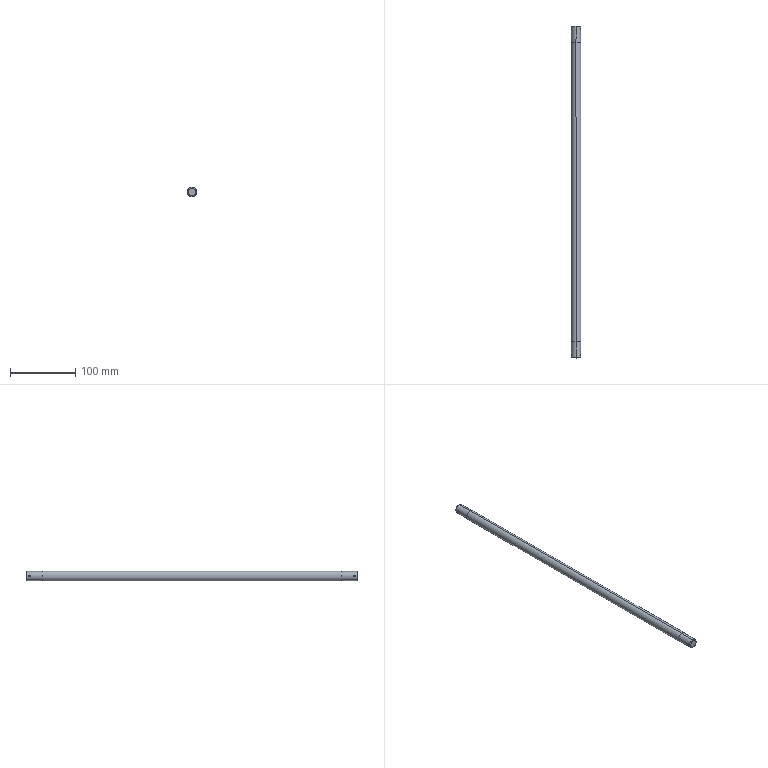Part | SolidWorks | features Chamfer 1, ICE 1, Revolution 1 | 1 solid | 18 faces | box 15 x 510 x 15 mm | volume 88747 mm3 | cylinder 10 | cone 4 | plane 4 | commonest cylinder face diameters 3 x4 14 x4 15 x2
STEP:
#1=CARTESIAN_POINT('',(-6.837,5.,1.5));
#2=VERTEX_POINT('',#1);
#3=CARTESIAN_POINT('',(-6.837,5.,-1.5));
#4=VERTEX_POINT('',#3);
#5=CARTESIAN_POINT('',(-6.837,5.,1.5));
#6=CARTESIAN_POINT('',(-6.837,4.804,1.5));
#7=CARTESIAN_POINT('',(-6.846,4.606,1.46));
#8=CARTESIAN_POINT('',(-6.877,4.245,1.311));
#9=CARTESIAN_POINT('',(-6.898,4.078,1.199));
#10=CARTESIAN_POINT('',(-6.93,3.871,0.9922));
#11=CARTESIAN_POINT('',(-6.94,3.808,0.9153));
#12=CARTESIAN_POINT('',(-6.96,3.699,0.753));
#13=CARTESIAN_POINT('',(-6.969,3.653,0.667));
#14=CARTESIAN_POINT('',(-6.991,3.539,0.3938));
#15=CARTESIAN_POINT('',(-7.,3.5,0.1987));
#16=CARTESIAN_POINT('',(-7.,3.5,-0.09833));
#17=CARTESIAN_POINT('',(-6.998,3.51,-0.1959));
#18=CARTESIAN_POINT('',(-6.99,3.548,-0.3882));
#19=CARTESIAN_POINT('',(-6.984,3.577,-0.4839));
#20=CARTESIAN_POINT('',(-6.961,3.689,-0.7556));
#21=CARTESIAN_POINT('',(-6.94,3.801,-0.9222));
#22=CARTESIAN_POINT('',(-6.898,4.076,-1.198));
#23=CARTESIAN_POINT('',(-6.877,4.243,-1.31));
#24=CARTESIAN_POINT('',(-6.846,4.604,-1.46));
#25=CARTESIAN_POINT('',(-6.837,4.801,-1.5));
#26=CARTESIAN_POINT('',(-6.837,5.,-1.5));
#27=B_SPLINE_CURVE_WITH_KNOTS('',3,(#5,#6,#7,#8,#9,#10,#11,#12,#13,#14,#15,#16,#17,#18,#19,#20,#21,#22,#23,#24,#25,#26),.UNSPECIFIED.,.F.,.F.,(4,2,2,2,2,2,2,2,2,2,4),(0.004703,0.005291,0.005879,0.006173,0.006467,0.007054,0.007348,0.007642,0.00823,0.008818,0.009405),.UNSPECIFIED.);
#28=EDGE_CURVE('',#2,#4,#27,.T.);
#29=ORIENTED_EDGE('',*,*,#28,.F.);
#30=CARTESIAN_POINT('',(6.837,5.,1.5));
#31=VERTEX_POINT('',#30);
#32=CARTESIAN_POINT('',(-7.5,5.,1.5));
#33=DIRECTION('',(1.,0.,0.));
#34=VECTOR('',#33,1000.);
#35=LINE('',#32,#34);
#36=EDGE_CURVE('',#2,#31,#35,.T.);
#37=ORIENTED_EDGE('',*,*,#36,.T.);
#38=CARTESIAN_POINT('',(6.837,5.,-1.5));
#39=VERTEX_POINT('',#38);
#40=CARTESIAN_POINT('',(6.837,5.,-1.5));
#41=CARTESIAN_POINT('',(6.837,4.901,-1.5));
#42=CARTESIAN_POINT('',(6.84,4.803,-1.49));
#43=CARTESIAN_POINT('',(6.848,4.611,-1.452));
#44=CARTESIAN_POINT('',(6.854,4.515,-1.423));
#45=CARTESIAN_POINT('',(6.869,4.334,-1.348));
#46=CARTESIAN_POINT('',(6.878,4.248,-1.301));
#47=CARTESIAN_POINT('',(6.898,4.085,-1.193));
#48=CARTESIAN_POINT('',(6.909,4.008,-1.129));
#49=CARTESIAN_POINT('',(6.94,3.801,-0.9225));
#50=CARTESIAN_POINT('',(6.961,3.69,-0.7555));
#51=CARTESIAN_POINT('',(6.991,3.54,-0.3947));
#52=CARTESIAN_POINT('',(7.,3.5,-0.1969));
#53=CARTESIAN_POINT('',(7.,3.5,0.09757));
#54=CARTESIAN_POINT('',(6.998,3.51,0.1973));
#55=CARTESIAN_POINT('',(6.99,3.548,0.3899));
#56=CARTESIAN_POINT('',(6.984,3.577,0.4836));
#57=CARTESIAN_POINT('',(6.961,3.69,0.7565));
#58=CARTESIAN_POINT('',(6.941,3.8,0.9216));
#59=CARTESIAN_POINT('',(6.908,4.009,1.13));
#60=CARTESIAN_POINT('',(6.898,4.085,1.192));
#61=CARTESIAN_POINT('',(6.878,4.247,1.301));
#62=CARTESIAN_POINT('',(6.869,4.335,1.348));
#63=CARTESIAN_POINT('',(6.854,4.516,1.423));
#64=CARTESIAN_POINT('',(6.848,4.609,1.452));
#65=CARTESIAN_POINT('',(6.84,4.802,1.49));
#66=CARTESIAN_POINT('',(6.837,4.902,1.5));
#67=CARTESIAN_POINT('',(6.837,5.,1.5));
#68=B_SPLINE_CURVE_WITH_KNOTS('',3,(#40,#41,#42,#43,#44,#45,#46,#47,#48,#49,#50,#51,#52,#53,#54,#55,#56,#57,#58,#59,#60,#61,#62,#63,#64,#65,#66,#67),.UNSPECIFIED.,.F.,.F.,(4,2,2,2,2,2,2,2,2,2,2,2,2,4),(0.,0.000294,0.0005879,0.0008819,0.001176,0.001764,0.002352,0.002646,0.00294,0.003527,0.003821,0.004115,0.004409,0.004703),.UNSPECIFIED.);
#69=EDGE_CURVE('',#39,#31,#68,.T.);
#70=ORIENTED_EDGE('',*,*,#69,.F.);
#71=CARTESIAN_POINT('',(-7.5,5.,-1.5));
#72=DIRECTION('',(1.,0.,0.));
#73=VECTOR('',#72,1000.);
#74=LINE('',#71,#73);
#75=EDGE_CURVE('',#4,#39,#74,.T.);
#76=ORIENTED_EDGE('',*,*,#75,.F.);
#77=EDGE_LOOP('',(#29,#37,#70,#76));
#78=FACE_OUTER_BOUND('',#77,.T.);
#79=CARTESIAN_POINT('',(-7.5,5.,0.));
#80=DIRECTION('',(1.,0.,0.));
#81=DIRECTION('',(0.,0.,-1.));
#82=AXIS2_PLACEMENT_3D('',#79,#80,#81);
#83=CYLINDRICAL_SURFACE('',#82,1.5);
#84=ADVANCED_FACE('',(#78),#83,.F.);
#85=CARTESIAN_POINT('',(-6.837,505.,1.5));
#86=VERTEX_POINT('',#85);
#87=CARTESIAN_POINT('',(-6.837,505.,-1.5));
#88=VERTEX_POINT('',#87);
#89=CARTESIAN_POINT('',(-6.837,505.,1.5));
#90=CARTESIAN_POINT('',(-6.837,504.804,1.5));
#91=CARTESIAN_POINT('',(-6.846,504.606,1.46));
#92=CARTESIAN_POINT('',(-6.877,504.245,1.311));
#93=CARTESIAN_POINT('',(-6.898,504.078,1.199));
#94=CARTESIAN_POINT('',(-6.93,503.871,0.9922));
#95=CARTESIAN_POINT('',(-6.94,503.808,0.9153));
#96=CARTESIAN_POINT('',(-6.96,503.699,0.753));
#97=CARTESIAN_POINT('',(-6.969,503.653,0.667));
#98=CARTESIAN_POINT('',(-6.991,503.539,0.3938));
#99=CARTESIAN_POINT('',(-7.,503.5,0.1987));
#100=CARTESIAN_POINT('',(-7.,503.5,-0.09833));
#101=CARTESIAN_POINT('',(-6.998,503.51,-0.1959));
#102=CARTESIAN_POINT('',(-6.99,503.548,-0.3882));
#103=CARTESIAN_POINT('',(-6.984,503.577,-0.4839));
#104=CARTESIAN_POINT('',(-6.961,503.689,-0.7556));
#105=CARTESIAN_POINT('',(-6.94,503.801,-0.9222));
#106=CARTESIAN_POINT('',(-6.898,504.076,-1.198));
#107=CARTESIAN_POINT('',(-6.877,504.243,-1.31));
#108=CARTESIAN_POINT('',(-6.846,504.604,-1.46));
#109=CARTESIAN_POINT('',(-6.837,504.801,-1.5));
#110=CARTESIAN_POINT('',(-6.837,505.,-1.5));
#111=B_SPLINE_CURVE_WITH_KNOTS('',3,(#89,#90,#91,#92,#93,#94,#95,#96,#97,#98,#99,#100,#101,#102,#103,#104,#105,#106,#107,#108,#109,#110),.UNSPECIFIED.,.F.,.F.,(4,2,2,2,2,2,2,2,2,2,4),(0.004703,0.005291,0.005879,0.006173,0.006467,0.007054,0.007348,0.007642,0.00823,0.008818,0.009405),.UNSPECIFIED.);
#112=EDGE_CURVE('',#86,#88,#111,.T.);
#113=ORIENTED_EDGE('',*,*,#112,.F.);
#114=CARTESIAN_POINT('',(6.837,505.,1.5));
#115=VERTEX_POINT('',#114);
#116=CARTESIAN_POINT('',(-7.5,505.,1.5));
#117=DIRECTION('',(1.,0.,0.));
#118=VECTOR('',#117,1000.);
#119=LINE('',#116,#118);
#120=EDGE_CURVE('',#86,#115,#119,.T.);
#121=ORIENTED_EDGE('',*,*,#120,.T.);
#122=CARTESIAN_POINT('',(6.837,505.,-1.5));
#123=VERTEX_POINT('',#122);
#124=CARTESIAN_POINT('',(6.837,505.,-1.5));
#125=CARTESIAN_POINT('',(6.837,504.901,-1.5));
#126=CARTESIAN_POINT('',(6.84,504.803,-1.49));
#127=CARTESIAN_POINT('',(6.848,504.611,-1.452));
#128=CARTESIAN_POINT('',(6.854,504.515,-1.423));
#129=CARTESIAN_POINT('',(6.869,504.334,-1.348));
#130=CARTESIAN_POINT('',(6.878,504.248,-1.301));
#131=CARTESIAN_POINT('',(6.898,504.085,-1.193));
#132=CARTESIAN_POINT('',(6.909,504.008,-1.129));
#133=CARTESIAN_POINT('',(6.94,503.801,-0.9225));
#134=CARTESIAN_POINT('',(6.961,503.69,-0.7555));
#135=CARTESIAN_POINT('',(6.991,503.54,-0.3947));
#136=CARTESIAN_POINT('',(7.,503.5,-0.1969));
#137=CARTESIAN_POINT('',(7.,503.5,0.09757));
#138=CARTESIAN_POINT('',(6.998,503.51,0.1973));
#139=CARTESIAN_POINT('',(6.99,503.548,0.3899));
#140=CARTESIAN_POINT('',(6.984,503.577,0.4836));
#141=CARTESIAN_POINT('',(6.961,503.69,0.7565));
#142=CARTESIAN_POINT('',(6.941,503.8,0.9216));
#143=CARTESIAN_POINT('',(6.908,504.009,1.13));
#144=CARTESIAN_POINT('',(6.898,504.085,1.192));
#145=CARTESIAN_POINT('',(6.878,504.247,1.301));
#146=CARTESIAN_POINT('',(6.869,504.335,1.348));
#147=CARTESIAN_POINT('',(6.854,504.516,1.423));
#148=CARTESIAN_POINT('',(6.848,504.609,1.452));
#149=CARTESIAN_POINT('',(6.84,504.802,1.49));
#150=CARTESIAN_POINT('',(6.837,504.902,1.5));
#151=CARTESIAN_POINT('',(6.837,505.,1.5));
#152=B_SPLINE_CURVE_WITH_KNOTS('',3,(#124,#125,#126,#127,#128,#129,#130,#131,#132,#133,#134,#135,#136,#137,#138,#139,#140,#141,#142,#143,#144,#145,#146,#147,#148,#149,#150,#151),.UNSPECIFIED.,.F.,.F.,(4,2,2,2,2,2,2,2,2,2,2,2,2,4),(0.,0.000294,0.0005879,0.0008819,0.001176,0.001764,0.002352,0.002646,0.00294,0.003527,0.003821,0.004115,0.004409,0.004703),.UNSPECIFIED.);
#153=EDGE_CURVE('',#123,#115,#152,.T.);
#154=ORIENTED_EDGE('',*,*,#153,.F.);
#155=CARTESIAN_POINT('',(-7.5,505.,-1.5));
#156=DIRECTION('',(1.,0.,0.));
#157=VECTOR('',#156,1000.);
#158=LINE('',#155,#157);
#159=EDGE_CURVE('',#88,#123,#158,.T.);
#160=ORIENTED_EDGE('',*,*,#159,.F.);
#161=EDGE_LOOP('',(#113,#121,#154,#160));
#162=FACE_OUTER_BOUND('',#161,.T.);
#163=CARTESIAN_POINT('',(-7.5,505.,0.));
#164=DIRECTION('',(1.,0.,0.));
#165=DIRECTION('',(0.,0.,-1.));
#166=AXIS2_PLACEMENT_3D('',#163,#164,#165);
#167=CYLINDRICAL_SURFACE('',#166,1.5);
#168=ADVANCED_FACE('',(#162),#167,.F.);
#169=CARTESIAN_POINT('',(0.,510.,6.));
#170=VERTEX_POINT('',#169);
#171=CARTESIAN_POINT('',(0.,510.,-6.));
#172=VERTEX_POINT('',#171);
#173=CARTESIAN_POINT('',(0.,510.,0.));
#174=DIRECTION('',(0.,1.,0.));
#175=DIRECTION('',(0.,0.,-1.));
#176=AXIS2_PLACEMENT_3D('',#173,#174,#175);
#177=CIRCLE('',#176,6.);
#178=EDGE_CURVE('',#170,#172,#177,.T.);
#179=ORIENTED_EDGE('',*,*,#178,.F.);
#180=CARTESIAN_POINT('',(0.,509.,7.));
#181=VERTEX_POINT('',#180);
#182=CARTESIAN_POINT('',(0.,510.,6.));
#183=DIRECTION('',(0.,-0.7071,0.7071));
#184=VECTOR('',#183,1000.);
#185=LINE('',#182,#184);
#186=EDGE_CURVE('',#170,#181,#185,.T.);
#187=ORIENTED_EDGE('',*,*,#186,.T.);
#188=CARTESIAN_POINT('',(0.,509.,-7.));
#189=VERTEX_POINT('',#188);
#190=CARTESIAN_POINT('',(0.,509.,0.));
#191=DIRECTION('',(0.,-1.,0.));
#192=DIRECTION('',(0.,0.,-1.));
#193=AXIS2_PLACEMENT_3D('',#190,#191,#192);
#194=CIRCLE('',#193,7.);
#195=EDGE_CURVE('',#189,#181,#194,.T.);
#196=ORIENTED_EDGE('',*,*,#195,.F.);
#197=CARTESIAN_POINT('',(0.,510.,-6.));
#198=DIRECTION('',(0.,-0.7071,-0.7071));
#199=VECTOR('',#198,1000.);
#200=LINE('',#197,#199);
#201=EDGE_CURVE('',#172,#189,#200,.T.);
#202=ORIENTED_EDGE('',*,*,#201,.F.);
#203=EDGE_LOOP('',(#179,#187,#196,#202));
#204=FACE_OUTER_BOUND('',#203,.T.);
#205=CARTESIAN_POINT('',(0.,510.,0.));
#206=DIRECTION('',(0.,-1.,0.));
#207=DIRECTION('',(0.,0.,-1.));
#208=AXIS2_PLACEMENT_3D('',#205,#206,#207);
#209=CONICAL_SURFACE('',#208,6.,0.7854);
#210=ADVANCED_FACE('',(#204),#209,.T.);
#211=CARTESIAN_POINT('',(0.,0.,-6.));
#212=VERTEX_POINT('',#211);
#213=CARTESIAN_POINT('',(0.,0.,6.));
#214=VERTEX_POINT('',#213);
#215=CARTESIAN_POINT('',(0.,0.,0.));
#216=DIRECTION('',(0.,-1.,0.));
#217=DIRECTION('',(0.,0.,1.));
#218=AXIS2_PLACEMENT_3D('',#215,#216,#217);
#219=CIRCLE('',#218,6.);
#220=EDGE_CURVE('',#212,#214,#219,.T.);
#221=ORIENTED_EDGE('',*,*,#220,.F.);
#222=CARTESIAN_POINT('',(0.,1.,-7.));
#223=VERTEX_POINT('',#222);
#224=CARTESIAN_POINT('',(0.,1.,-7.));
#225=DIRECTION('',(0.,0.7071,-0.7071));
#226=VECTOR('',#225,1000.);
#227=LINE('',#224,#226);
#228=EDGE_CURVE('',#212,#223,#227,.T.);
#229=ORIENTED_EDGE('',*,*,#228,.T.);
#230=CARTESIAN_POINT('',(0.,1.,7.));
#231=VERTEX_POINT('',#230);
#232=CARTESIAN_POINT('',(0.,1.,0.));
#233=DIRECTION('',(0.,1.,0.));
#234=DIRECTION('',(0.,0.,1.));
#235=AXIS2_PLACEMENT_3D('',#232,#233,#234);
#236=CIRCLE('',#235,7.);
#237=EDGE_CURVE('',#231,#223,#236,.T.);
#238=ORIENTED_EDGE('',*,*,#237,.F.);
#239=CARTESIAN_POINT('',(0.,1.,7.));
#240=DIRECTION('',(0.,0.7071,0.7071));
#241=VECTOR('',#240,1000.);
#242=LINE('',#239,#241);
#243=EDGE_CURVE('',#214,#231,#242,.T.);
#244=ORIENTED_EDGE('',*,*,#243,.F.);
#245=EDGE_LOOP('',(#221,#229,#238,#244));
#246=FACE_OUTER_BOUND('',#245,.T.);
#247=CARTESIAN_POINT('',(0.,1.,0.));
#248=DIRECTION('',(0.,1.,0.));
#249=DIRECTION('',(0.,0.,1.));
#250=AXIS2_PLACEMENT_3D('',#247,#248,#249);
#251=CONICAL_SURFACE('',#250,7.,0.7854);
#252=ADVANCED_FACE('',(#246),#251,.T.);
#253=ORIENTED_EDGE('',*,*,#153,.T.);
#254=CARTESIAN_POINT('',(6.837,505.,1.5));
#255=CARTESIAN_POINT('',(6.837,505.196,1.5));
#256=CARTESIAN_POINT('',(6.846,505.394,1.46));
#257=CARTESIAN_POINT('',(6.877,505.755,1.311));
#258=CARTESIAN_POINT('',(6.898,505.922,1.199));
#259=CARTESIAN_POINT('',(6.93,506.129,0.9922));
#260=CARTESIAN_POINT('',(6.94,506.192,0.9153));
#261=CARTESIAN_POINT('',(6.96,506.301,0.753));
#262=CARTESIAN_POINT('',(6.969,506.347,0.667));
#263=CARTESIAN_POINT('',(6.991,506.461,0.3938));
#264=CARTESIAN_POINT('',(7.,506.5,0.1987));
#265=CARTESIAN_POINT('',(7.,506.5,-0.09833));
#266=CARTESIAN_POINT('',(6.998,506.49,-0.1959));
#267=CARTESIAN_POINT('',(6.99,506.452,-0.3882));
#268=CARTESIAN_POINT('',(6.984,506.423,-0.4839));
#269=CARTESIAN_POINT('',(6.961,506.311,-0.7556));
#270=CARTESIAN_POINT('',(6.94,506.199,-0.9222));
#271=CARTESIAN_POINT('',(6.898,505.924,-1.198));
#272=CARTESIAN_POINT('',(6.877,505.757,-1.31));
#273=CARTESIAN_POINT('',(6.846,505.396,-1.46));
#274=CARTESIAN_POINT('',(6.837,505.199,-1.5));
#275=CARTESIAN_POINT('',(6.837,505.,-1.5));
#276=B_SPLINE_CURVE_WITH_KNOTS('',3,(#254,#255,#256,#257,#258,#259,#260,#261,#262,#263,#264,#265,#266,#267,#268,#269,#270,#271,#272,#273,#274,#275),.UNSPECIFIED.,.F.,.F.,(4,2,2,2,2,2,2,2,2,2,4),(0.004703,0.005291,0.005879,0.006173,0.006467,0.007054,0.007348,0.007642,0.00823,0.008818,0.009405),.UNSPECIFIED.);
#277=EDGE_CURVE('',#115,#123,#276,.T.);
#278=ORIENTED_EDGE('',*,*,#277,.T.);
#279=EDGE_LOOP('',(#253,#278));
#280=FACE_BOUND('',#279,.T.);
#281=CARTESIAN_POINT('',(0.,485.,7.));
#282=VERTEX_POINT('',#281);
#283=CARTESIAN_POINT('',(0.,485.,-7.));
#284=VERTEX_POINT('',#283);
#285=CARTESIAN_POINT('',(0.,485.,0.));
#286=DIRECTION('',(0.,1.,0.));
#287=DIRECTION('',(0.,0.,1.));
#288=AXIS2_PLACEMENT_3D('',#285,#286,#287);
#289=CIRCLE('',#288,7.);
#290=EDGE_CURVE('',#282,#284,#289,.T.);
#291=ORIENTED_EDGE('',*,*,#290,.T.);
#292=CARTESIAN_POINT('',(0.,0.,-7.));
#293=DIRECTION('',(0.,1.,0.));
#294=VECTOR('',#293,1000.);
#295=LINE('',#292,#294);
#296=EDGE_CURVE('',#284,#189,#295,.T.);
#297=ORIENTED_EDGE('',*,*,#296,.T.);
#298=ORIENTED_EDGE('',*,*,#195,.T.);
#299=CARTESIAN_POINT('',(0.,0.,7.));
#300=DIRECTION('',(0.,1.,0.));
#301=VECTOR('',#300,1000.);
#302=LINE('',#299,#301);
#303=EDGE_CURVE('',#282,#181,#302,.T.);
#304=ORIENTED_EDGE('',*,*,#303,.F.);
#305=EDGE_LOOP('',(#291,#297,#298,#304));
#306=FACE_OUTER_BOUND('',#305,.T.);
#307=CARTESIAN_POINT('',(0.,0.,0.));
#308=DIRECTION('',(0.,1.,0.));
#309=DIRECTION('',(0.,0.,1.));
#310=AXIS2_PLACEMENT_3D('',#307,#308,#309);
#311=CYLINDRICAL_SURFACE('',#310,7.);
#312=ADVANCED_FACE('',(#280,#306),#311,.T.);
#313=CARTESIAN_POINT('',(0.,25.,7.5));
#314=VERTEX_POINT('',#313);
#315=CARTESIAN_POINT('',(0.,25.,-7.5));
#316=VERTEX_POINT('',#315);
#317=CARTESIAN_POINT('',(0.,25.,0.));
#318=DIRECTION('',(0.,1.,0.));
#319=DIRECTION('',(0.,0.,1.));
#320=AXIS2_PLACEMENT_3D('',#317,#318,#319);
#321=CIRCLE('',#320,7.5);
#322=EDGE_CURVE('',#314,#316,#321,.T.);
#323=ORIENTED_EDGE('',*,*,#322,.T.);
#324=CARTESIAN_POINT('',(0.,485.,-7.5));
#325=VERTEX_POINT('',#324);
#326=CARTESIAN_POINT('',(0.,0.,-7.5));
#327=DIRECTION('',(0.,1.,0.));
#328=VECTOR('',#327,1000.);
#329=LINE('',#326,#328);
#330=EDGE_CURVE('',#316,#325,#329,.T.);
#331=ORIENTED_EDGE('',*,*,#330,.T.);
#332=CARTESIAN_POINT('',(0.,485.,7.5));
#333=VERTEX_POINT('',#332);
#334=CARTESIAN_POINT('',(0.,485.,0.));
#335=DIRECTION('',(0.,1.,0.));
#336=DIRECTION('',(0.,0.,1.));
#337=AXIS2_PLACEMENT_3D('',#334,#335,#336);
#338=CIRCLE('',#337,7.5);
#339=EDGE_CURVE('',#333,#325,#338,.T.);
#340=ORIENTED_EDGE('',*,*,#339,.F.);
#341=CARTESIAN_POINT('',(0.,0.,7.5));
#342=DIRECTION('',(0.,1.,0.));
#343=VECTOR('',#342,1000.);
#344=LINE('',#341,#343);
#345=EDGE_CURVE('',#314,#333,#344,.T.);
#346=ORIENTED_EDGE('',*,*,#345,.F.);
#347=EDGE_LOOP('',(#323,#331,#340,#346));
#348=FACE_OUTER_BOUND('',#347,.T.);
#349=CARTESIAN_POINT('',(0.,0.,0.));
#350=DIRECTION('',(0.,1.,0.));
#351=DIRECTION('',(0.,0.,1.));
#352=AXIS2_PLACEMENT_3D('',#349,#350,#351);
#353=CYLINDRICAL_SURFACE('',#352,7.5);
#354=ADVANCED_FACE('',(#348),#353,.T.);
#355=ORIENTED_EDGE('',*,*,#69,.T.);
#356=CARTESIAN_POINT('',(6.837,5.,1.5));
#357=CARTESIAN_POINT('',(6.837,5.196,1.5));
#358=CARTESIAN_POINT('',(6.846,5.394,1.46));
#359=CARTESIAN_POINT('',(6.877,5.755,1.311));
#360=CARTESIAN_POINT('',(6.898,5.922,1.199));
#361=CARTESIAN_POINT('',(6.93,6.129,0.9922));
#362=CARTESIAN_POINT('',(6.94,6.192,0.9153));
#363=CARTESIAN_POINT('',(6.96,6.301,0.753));
#364=CARTESIAN_POINT('',(6.969,6.347,0.667));
#365=CARTESIAN_POINT('',(6.991,6.461,0.3938));
#366=CARTESIAN_POINT('',(7.,6.5,0.1987));
#367=CARTESIAN_POINT('',(7.,6.5,-0.09833));
#368=CARTESIAN_POINT('',(6.998,6.49,-0.1959));
#369=CARTESIAN_POINT('',(6.99,6.452,-0.3882));
#370=CARTESIAN_POINT('',(6.984,6.423,-0.4839));
#371=CARTESIAN_POINT('',(6.961,6.311,-0.7556));
#372=CARTESIAN_POINT('',(6.94,6.199,-0.9222));
#373=CARTESIAN_POINT('',(6.898,5.924,-1.198));
#374=CARTESIAN_POINT('',(6.877,5.757,-1.31));
#375=CARTESIAN_POINT('',(6.846,5.396,-1.46));
#376=CARTESIAN_POINT('',(6.837,5.199,-1.5));
#377=CARTESIAN_POINT('',(6.837,5.,-1.5));
#378=B_SPLINE_CURVE_WITH_KNOTS('',3,(#356,#357,#358,#359,#360,#361,#362,#363,#364,#365,#366,#367,#368,#369,#370,#371,#372,#373,#374,#375,#376,#377),.UNSPECIFIED.,.F.,.F.,(4,2,2,2,2,2,2,2,2,2,4),(0.004703,0.005291,0.005879,0.006173,0.006467,0.007054,0.007348,0.007642,0.00823,0.008818,0.009405),.UNSPECIFIED.);
#379=EDGE_CURVE('',#31,#39,#378,.T.);
#380=ORIENTED_EDGE('',*,*,#379,.T.);
#381=EDGE_LOOP('',(#355,#380));
#382=FACE_BOUND('',#381,.T.);
#383=ORIENTED_EDGE('',*,*,#237,.T.);
#384=CARTESIAN_POINT('',(0.,25.,-7.));
#385=VERTEX_POINT('',#384);
#386=CARTESIAN_POINT('',(0.,0.,-7.));
#387=DIRECTION('',(0.,1.,0.));
#388=VECTOR('',#387,1000.);
#389=LINE('',#386,#388);
#390=EDGE_CURVE('',#223,#385,#389,.T.);
#391=ORIENTED_EDGE('',*,*,#390,.T.);
#392=CARTESIAN_POINT('',(0.,25.,7.));
#393=VERTEX_POINT('',#392);
#394=CARTESIAN_POINT('',(0.,25.,0.));
#395=DIRECTION('',(0.,1.,0.));
#396=DIRECTION('',(0.,0.,1.));
#397=AXIS2_PLACEMENT_3D('',#394,#395,#396);
#398=CIRCLE('',#397,7.);
#399=EDGE_CURVE('',#393,#385,#398,.T.);
#400=ORIENTED_EDGE('',*,*,#399,.F.);
#401=CARTESIAN_POINT('',(0.,0.,7.));
#402=DIRECTION('',(0.,1.,0.));
#403=VECTOR('',#402,1000.);
#404=LINE('',#401,#403);
#405=EDGE_CURVE('',#231,#393,#404,.T.);
#406=ORIENTED_EDGE('',*,*,#405,.F.);
#407=EDGE_LOOP('',(#383,#391,#400,#406));
#408=FACE_OUTER_BOUND('',#407,.T.);
#409=CARTESIAN_POINT('',(0.,0.,0.));
#410=DIRECTION('',(0.,1.,0.));
#411=DIRECTION('',(0.,0.,1.));
#412=AXIS2_PLACEMENT_3D('',#409,#410,#411);
#413=CYLINDRICAL_SURFACE('',#412,7.);
#414=ADVANCED_FACE('',(#382,#408),#413,.T.);
#415=CARTESIAN_POINT('',(0.,0.,0.));
#416=DIRECTION('',(0.,-1.,0.));
#417=DIRECTION('',(0.,0.,1.));
#418=AXIS2_PLACEMENT_3D('',#415,#416,#417);
#419=CIRCLE('',#418,6.);
#420=EDGE_CURVE('',#214,#212,#419,.T.);
#421=ORIENTED_EDGE('',*,*,#420,.T.);
#422=ORIENTED_EDGE('',*,*,#220,.T.);
#423=EDGE_LOOP('',(#421,#422));
#424=FACE_OUTER_BOUND('',#423,.T.);
#425=CARTESIAN_POINT('',(0.,0.,0.));
#426=DIRECTION('',(0.,1.,0.));
#427=DIRECTION('',(0.,0.,1.));
#428=AXIS2_PLACEMENT_3D('',#425,#426,#427);
#429=PLANE('',#428);
#430=ADVANCED_FACE('',(#424),#429,.F.);
#431=ORIENTED_EDGE('',*,*,#390,.F.);
#432=CARTESIAN_POINT('',(0.,1.,0.));
#433=DIRECTION('',(0.,1.,0.));
#434=DIRECTION('',(0.,0.,1.));
#435=AXIS2_PLACEMENT_3D('',#432,#433,#434);
#436=CIRCLE('',#435,7.);
#437=EDGE_CURVE('',#223,#231,#436,.T.);
#438=ORIENTED_EDGE('',*,*,#437,.T.);
#439=ORIENTED_EDGE('',*,*,#405,.T.);
#440=CARTESIAN_POINT('',(0.,25.,0.));
#441=DIRECTION('',(0.,1.,0.));
#442=DIRECTION('',(0.,0.,1.));
#443=AXIS2_PLACEMENT_3D('',#440,#441,#442);
#444=CIRCLE('',#443,7.);
#445=EDGE_CURVE('',#385,#393,#444,.T.);
#446=ORIENTED_EDGE('',*,*,#445,.F.);
#447=EDGE_LOOP('',(#431,#438,#439,#446));
#448=FACE_OUTER_BOUND('',#447,.T.);
#449=CARTESIAN_POINT('',(-6.837,5.,-1.5));
#450=CARTESIAN_POINT('',(-6.837,5.099,-1.5));
#451=CARTESIAN_POINT('',(-6.84,5.197,-1.49));
#452=CARTESIAN_POINT('',(-6.848,5.389,-1.452));
#453=CARTESIAN_POINT('',(-6.854,5.485,-1.423));
#454=CARTESIAN_POINT('',(-6.869,5.666,-1.348));
#455=CARTESIAN_POINT('',(-6.878,5.752,-1.301));
#456=CARTESIAN_POINT('',(-6.898,5.915,-1.193));
#457=CARTESIAN_POINT('',(-6.909,5.992,-1.129));
#458=CARTESIAN_POINT('',(-6.94,6.199,-0.9225));
#459=CARTESIAN_POINT('',(-6.961,6.31,-0.7555));
#460=CARTESIAN_POINT('',(-6.991,6.46,-0.3947));
#461=CARTESIAN_POINT('',(-7.,6.5,-0.1969));
#462=CARTESIAN_POINT('',(-7.,6.5,0.09757));
#463=CARTESIAN_POINT('',(-6.998,6.49,0.1973));
#464=CARTESIAN_POINT('',(-6.99,6.452,0.3899));
#465=CARTESIAN_POINT('',(-6.984,6.423,0.4836));
#466=CARTESIAN_POINT('',(-6.961,6.31,0.7565));
#467=CARTESIAN_POINT('',(-6.941,6.2,0.9216));
#468=CARTESIAN_POINT('',(-6.908,5.991,1.13));
#469=CARTESIAN_POINT('',(-6.898,5.915,1.192));
#470=CARTESIAN_POINT('',(-6.878,5.753,1.301));
#471=CARTESIAN_POINT('',(-6.869,5.665,1.348));
#472=CARTESIAN_POINT('',(-6.854,5.484,1.423));
#473=CARTESIAN_POINT('',(-6.848,5.391,1.452));
#474=CARTESIAN_POINT('',(-6.84,5.198,1.49));
#475=CARTESIAN_POINT('',(-6.837,5.098,1.5));
#476=CARTESIAN_POINT('',(-6.837,5.,1.5));
#477=B_SPLINE_CURVE_WITH_KNOTS('',3,(#449,#450,#451,#452,#453,#454,#455,#456,#457,#458,#459,#460,#461,#462,#463,#464,#465,#466,#467,#468,#469,#470,#471,#472,#473,#474,#475,#476),.UNSPECIFIED.,.F.,.F.,(4,2,2,2,2,2,2,2,2,2,2,2,2,4),(0.,0.000294,0.0005879,0.0008819,0.001176,0.001764,0.002352,0.002646,0.00294,0.003527,0.003821,0.004115,0.004409,0.004703),.UNSPECIFIED.);
#478=EDGE_CURVE('',#4,#2,#477,.T.);
#479=ORIENTED_EDGE('',*,*,#478,.T.);
#480=ORIENTED_EDGE('',*,*,#28,.T.);
#481=EDGE_LOOP('',(#479,#480));
#482=FACE_BOUND('',#481,.T.);
#483=CARTESIAN_POINT('',(0.,0.,0.));
#484=DIRECTION('',(0.,1.,0.));
#485=DIRECTION('',(0.,0.,1.));
#486=AXIS2_PLACEMENT_3D('',#483,#484,#485);
#487=CYLINDRICAL_SURFACE('',#486,7.);
#488=ADVANCED_FACE('',(#448,#482),#487,.T.);
#489=ORIENTED_EDGE('',*,*,#322,.F.);
#490=CARTESIAN_POINT('',(0.,25.,0.));
#491=DIRECTION('',(0.,1.,0.));
#492=DIRECTION('',(0.,0.,1.));
#493=AXIS2_PLACEMENT_3D('',#490,#491,#492);
#494=CIRCLE('',#493,7.5);
#495=EDGE_CURVE('',#316,#314,#494,.T.);
#496=ORIENTED_EDGE('',*,*,#495,.F.);
#497=EDGE_LOOP('',(#489,#496));
#498=FACE_OUTER_BOUND('',#497,.T.);
#499=ORIENTED_EDGE('',*,*,#399,.T.);
#500=ORIENTED_EDGE('',*,*,#445,.T.);
#501=EDGE_LOOP('',(#499,#500));
#502=FACE_BOUND('',#501,.T.);
#503=CARTESIAN_POINT('',(7.,25.,0.));
#504=DIRECTION('',(0.,1.,0.));
#505=DIRECTION('',(0.,0.,1.));
#506=AXIS2_PLACEMENT_3D('',#503,#504,#505);
#507=PLANE('',#506);
#508=ADVANCED_FACE('',(#498,#502),#507,.F.);
#509=ORIENTED_EDGE('',*,*,#330,.F.);
#510=ORIENTED_EDGE('',*,*,#495,.T.);
#511=ORIENTED_EDGE('',*,*,#345,.T.);
#512=CARTESIAN_POINT('',(0.,485.,0.));
#513=DIRECTION('',(0.,1.,0.));
#514=DIRECTION('',(0.,0.,1.));
#515=AXIS2_PLACEMENT_3D('',#512,#513,#514);
#516=CIRCLE('',#515,7.5);
#517=EDGE_CURVE('',#325,#333,#516,.T.);
#518=ORIENTED_EDGE('',*,*,#517,.F.);
#519=EDGE_LOOP('',(#509,#510,#511,#518));
#520=FACE_OUTER_BOUND('',#519,.T.);
#521=CARTESIAN_POINT('',(0.,0.,0.));
#522=DIRECTION('',(0.,1.,0.));
#523=DIRECTION('',(0.,0.,1.));
#524=AXIS2_PLACEMENT_3D('',#521,#522,#523);
#525=CYLINDRICAL_SURFACE('',#524,7.5);
#526=ADVANCED_FACE('',(#520),#525,.T.);
#527=ORIENTED_EDGE('',*,*,#290,.F.);
#528=CARTESIAN_POINT('',(0.,485.,0.));
#529=DIRECTION('',(0.,1.,0.));
#530=DIRECTION('',(0.,0.,1.));
#531=AXIS2_PLACEMENT_3D('',#528,#529,#530);
#532=CIRCLE('',#531,7.);
#533=EDGE_CURVE('',#284,#282,#532,.T.);
#534=ORIENTED_EDGE('',*,*,#533,.F.);
#535=EDGE_LOOP('',(#527,#534));
#536=FACE_BOUND('',#535,.T.);
#537=ORIENTED_EDGE('',*,*,#339,.T.);
#538=ORIENTED_EDGE('',*,*,#517,.T.);
#539=EDGE_LOOP('',(#537,#538));
#540=FACE_OUTER_BOUND('',#539,.T.);
#541=CARTESIAN_POINT('',(7.5,485.,0.));
#542=DIRECTION('',(0.,-1.,0.));
#543=DIRECTION('',(0.,0.,-1.));
#544=AXIS2_PLACEMENT_3D('',#541,#542,#543);
#545=PLANE('',#544);
#546=ADVANCED_FACE('',(#536,#540),#545,.F.);
#547=ORIENTED_EDGE('',*,*,#296,.F.);
#548=ORIENTED_EDGE('',*,*,#533,.T.);
#549=ORIENTED_EDGE('',*,*,#303,.T.);
#550=CARTESIAN_POINT('',(0.,509.,0.));
#551=DIRECTION('',(0.,-1.,0.));
#552=DIRECTION('',(0.,0.,-1.));
#553=AXIS2_PLACEMENT_3D('',#550,#551,#552);
#554=CIRCLE('',#553,7.);
#555=EDGE_CURVE('',#181,#189,#554,.T.);
#556=ORIENTED_EDGE('',*,*,#555,.T.);
#557=EDGE_LOOP('',(#547,#548,#549,#556));
#558=FACE_OUTER_BOUND('',#557,.T.);
#559=CARTESIAN_POINT('',(-6.837,505.,-1.5));
#560=CARTESIAN_POINT('',(-6.837,505.099,-1.5));
#561=CARTESIAN_POINT('',(-6.84,505.197,-1.49));
#562=CARTESIAN_POINT('',(-6.848,505.389,-1.452));
#563=CARTESIAN_POINT('',(-6.854,505.485,-1.423));
#564=CARTESIAN_POINT('',(-6.869,505.666,-1.348));
#565=CARTESIAN_POINT('',(-6.878,505.752,-1.301));
#566=CARTESIAN_POINT('',(-6.898,505.915,-1.193));
#567=CARTESIAN_POINT('',(-6.909,505.992,-1.129));
#568=CARTESIAN_POINT('',(-6.94,506.199,-0.9225));
#569=CARTESIAN_POINT('',(-6.961,506.31,-0.7555));
#570=CARTESIAN_POINT('',(-6.991,506.46,-0.3947));
#571=CARTESIAN_POINT('',(-7.,506.5,-0.1969));
#572=CARTESIAN_POINT('',(-7.,506.5,0.09757));
#573=CARTESIAN_POINT('',(-6.998,506.49,0.1973));
#574=CARTESIAN_POINT('',(-6.99,506.452,0.3899));
#575=CARTESIAN_POINT('',(-6.984,506.423,0.4836));
#576=CARTESIAN_POINT('',(-6.961,506.31,0.7565));
#577=CARTESIAN_POINT('',(-6.941,506.2,0.9216));
#578=CARTESIAN_POINT('',(-6.908,505.991,1.13));
#579=CARTESIAN_POINT('',(-6.898,505.915,1.192));
#580=CARTESIAN_POINT('',(-6.878,505.753,1.301));
#581=CARTESIAN_POINT('',(-6.869,505.665,1.348));
#582=CARTESIAN_POINT('',(-6.854,505.484,1.423));
#583=CARTESIAN_POINT('',(-6.848,505.391,1.452));
#584=CARTESIAN_POINT('',(-6.84,505.198,1.49));
#585=CARTESIAN_POINT('',(-6.837,505.098,1.5));
#586=CARTESIAN_POINT('',(-6.837,505.,1.5));
#587=B_SPLINE_CURVE_WITH_KNOTS('',3,(#559,#560,#561,#562,#563,#564,#565,#566,#567,#568,#569,#570,#571,#572,#573,#574,#575,#576,#577,#578,#579,#580,#581,#582,#583,#584,#585,#586),.UNSPECIFIED.,.F.,.F.,(4,2,2,2,2,2,2,2,2,2,2,2,2,4),(0.,0.000294,0.0005879,0.0008819,0.001176,0.001764,0.002352,0.002646,0.00294,0.003527,0.003821,0.004115,0.004409,0.004703),.UNSPECIFIED.);
#588=EDGE_CURVE('',#88,#86,#587,.T.);
#589=ORIENTED_EDGE('',*,*,#588,.T.);
#590=ORIENTED_EDGE('',*,*,#112,.T.);
#591=EDGE_LOOP('',(#589,#590));
#592=FACE_BOUND('',#591,.T.);
#593=CARTESIAN_POINT('',(0.,0.,0.));
#594=DIRECTION('',(0.,1.,0.));
#595=DIRECTION('',(0.,0.,1.));
#596=AXIS2_PLACEMENT_3D('',#593,#594,#595);
#597=CYLINDRICAL_SURFACE('',#596,7.);
#598=ADVANCED_FACE('',(#558,#592),#597,.T.);
#599=CARTESIAN_POINT('',(0.,510.,0.));
#600=DIRECTION('',(0.,1.,0.));
#601=DIRECTION('',(0.,0.,-1.));
#602=AXIS2_PLACEMENT_3D('',#599,#600,#601);
#603=CIRCLE('',#602,6.);
#604=EDGE_CURVE('',#172,#170,#603,.T.);
#605=ORIENTED_EDGE('',*,*,#604,.T.);
#606=ORIENTED_EDGE('',*,*,#178,.T.);
#607=EDGE_LOOP('',(#605,#606));
#608=FACE_OUTER_BOUND('',#607,.T.);
#609=CARTESIAN_POINT('',(7.,510.,0.));
#610=DIRECTION('',(0.,-1.,0.));
#611=DIRECTION('',(0.,0.,-1.));
#612=AXIS2_PLACEMENT_3D('',#609,#610,#611);
#613=PLANE('',#612);
#614=ADVANCED_FACE('',(#608),#613,.F.);
#615=ORIENTED_EDGE('',*,*,#228,.F.);
#616=ORIENTED_EDGE('',*,*,#420,.F.);
#617=ORIENTED_EDGE('',*,*,#243,.T.);
#618=ORIENTED_EDGE('',*,*,#437,.F.);
#619=EDGE_LOOP('',(#615,#616,#617,#618));
#620=FACE_OUTER_BOUND('',#619,.T.);
#621=CARTESIAN_POINT('',(0.,1.,0.));
#622=DIRECTION('',(0.,1.,0.));
#623=DIRECTION('',(0.,0.,1.));
#624=AXIS2_PLACEMENT_3D('',#621,#622,#623);
#625=CONICAL_SURFACE('',#624,7.,0.7854);
#626=ADVANCED_FACE('',(#620),#625,.T.);
#627=ORIENTED_EDGE('',*,*,#186,.F.);
#628=ORIENTED_EDGE('',*,*,#604,.F.);
#629=ORIENTED_EDGE('',*,*,#201,.T.);
#630=ORIENTED_EDGE('',*,*,#555,.F.);
#631=EDGE_LOOP('',(#627,#628,#629,#630));
#632=FACE_OUTER_BOUND('',#631,.T.);
#633=CARTESIAN_POINT('',(0.,510.,0.));
#634=DIRECTION('',(0.,-1.,0.));
#635=DIRECTION('',(0.,0.,-1.));
#636=AXIS2_PLACEMENT_3D('',#633,#634,#635);
#637=CONICAL_SURFACE('',#636,6.,0.7854);
#638=ADVANCED_FACE('',(#632),#637,.T.);
#639=ORIENTED_EDGE('',*,*,#120,.F.);
#640=ORIENTED_EDGE('',*,*,#588,.F.);
#641=ORIENTED_EDGE('',*,*,#159,.T.);
#642=ORIENTED_EDGE('',*,*,#277,.F.);
#643=EDGE_LOOP('',(#639,#640,#641,#642));
#644=FACE_OUTER_BOUND('',#643,.T.);
#645=CARTESIAN_POINT('',(-7.5,505.,0.));
#646=DIRECTION('',(1.,0.,0.));
#647=DIRECTION('',(0.,0.,-1.));
#648=AXIS2_PLACEMENT_3D('',#645,#646,#647);
#649=CYLINDRICAL_SURFACE('',#648,1.5);
#650=ADVANCED_FACE('',(#644),#649,.F.);
#651=ORIENTED_EDGE('',*,*,#36,.F.);
#652=ORIENTED_EDGE('',*,*,#478,.F.);
#653=ORIENTED_EDGE('',*,*,#75,.T.);
#654=ORIENTED_EDGE('',*,*,#379,.F.);
#655=EDGE_LOOP('',(#651,#652,#653,#654));
#656=FACE_OUTER_BOUND('',#655,.T.);
#657=CARTESIAN_POINT('',(-7.5,5.,0.));
#658=DIRECTION('',(1.,0.,0.));
#659=DIRECTION('',(0.,0.,-1.));
#660=AXIS2_PLACEMENT_3D('',#657,#658,#659);
#661=CYLINDRICAL_SURFACE('',#660,1.5);
#662=ADVANCED_FACE('',(#656),#661,.F.);
#663=CLOSED_SHELL('',(#84,#168,#210,#252,#312,#354,#414,#430,#488,#508,#526,#546,#598,#614,#626,#638,#650,#662));
#664=MANIFOLD_SOLID_BREP('',#663);
#665=CARTESIAN_POINT('',(0.,0.,0.));
#666=DIRECTION('',(0.,0.,1.));
#667=DIRECTION('',(1.,0.,0.));
#668=AXIS2_PLACEMENT_3D('',#665,#666,#667);
#669=(LENGTH_UNIT()NAMED_UNIT(*)SI_UNIT(.MILLI.,.METRE.));
#670=UNCERTAINTY_MEASURE_WITH_UNIT(LENGTH_MEASURE(0.00001),#669,'','');
#671=(NAMED_UNIT(*)PLANE_ANGLE_UNIT()SI_UNIT($,.RADIAN.));
#672=(NAMED_UNIT(*)SI_UNIT($,.STERADIAN.)SOLID_ANGLE_UNIT());
#673=(GEOMETRIC_REPRESENTATION_CONTEXT(3)GLOBAL_UNCERTAINTY_ASSIGNED_CONTEXT((#670))GLOBAL_UNIT_ASSIGNED_CONTEXT((#669,#671,#672))REPRESENTATION_CONTEXT('',''));
#674=ADVANCED_BREP_SHAPE_REPRESENTATION('',(#664,#668),#673);